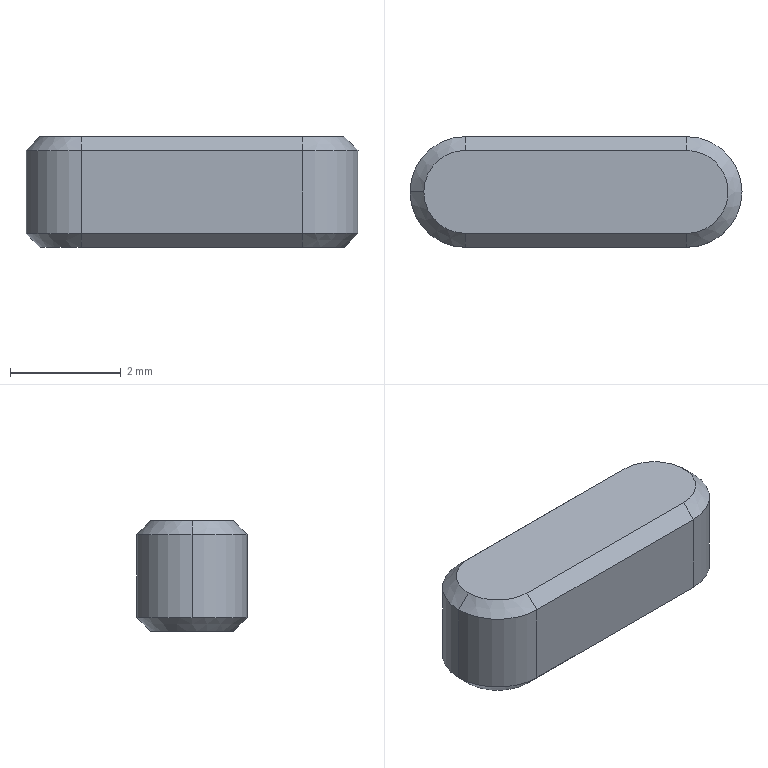Part | SolidWorks | features BaseBody 1 | 1 solid | 17 faces | box 6 x 2 x 2 mm | volume 21.423 mm3 | plane 8 | cone 6 | cylinder 3 | commonest cylinder face diameters 2 x3
STEP:
#1=CARTESIAN_POINT('',(-4.,-0.75,1.));
#2=VERTEX_POINT('',#1);
#3=CARTESIAN_POINT('',(-4.75,0.,1.));
#4=VERTEX_POINT('',#3);
#5=CARTESIAN_POINT('',(-4.,0.,1.));
#6=DIRECTION('',(0.,0.,-1.));
#7=DIRECTION('',(-1.,0.,0.));
#8=AXIS2_PLACEMENT_3D('',#5,#6,#7);
#9=CIRCLE('',#8,0.75);
#10=EDGE_CURVE('',#2,#4,#9,.T.);
#11=ORIENTED_EDGE('',*,*,#10,.T.);
#12=CARTESIAN_POINT('',(-5.,0.,0.75));
#13=VERTEX_POINT('',#12);
#14=CARTESIAN_POINT('',(-5.,0.,0.75));
#15=DIRECTION('',(-0.7071,0.,-0.7071));
#16=VECTOR('',#15,1000.);
#17=LINE('',#14,#16);
#18=EDGE_CURVE('',#4,#13,#17,.T.);
#19=ORIENTED_EDGE('',*,*,#18,.T.);
#20=CARTESIAN_POINT('',(-4.,-1.,0.75));
#21=VERTEX_POINT('',#20);
#22=CARTESIAN_POINT('',(-4.,0.,0.75));
#23=DIRECTION('',(0.,0.,1.));
#24=DIRECTION('',(-1.,0.,0.));
#25=AXIS2_PLACEMENT_3D('',#22,#23,#24);
#26=CIRCLE('',#25,1.);
#27=EDGE_CURVE('',#13,#21,#26,.T.);
#28=ORIENTED_EDGE('',*,*,#27,.T.);
#29=CARTESIAN_POINT('',(-4.,-498996.,-498994.25));
#30=DIRECTION('',(0.,0.7071,0.7071));
#31=VECTOR('',#30,1000.);
#32=LINE('',#29,#31);
#33=EDGE_CURVE('',#21,#2,#32,.T.);
#34=ORIENTED_EDGE('',*,*,#33,.T.);
#35=EDGE_LOOP('',(#11,#19,#28,#34));
#36=FACE_OUTER_BOUND('',#35,.T.);
#37=CARTESIAN_POINT('',(-4.,0.,0.75));
#38=DIRECTION('',(0.,0.,-1.));
#39=DIRECTION('',(-1.,0.,0.));
#40=AXIS2_PLACEMENT_3D('',#37,#38,#39);
#41=CONICAL_SURFACE('',#40,1.,0.7854);
#42=ADVANCED_FACE('',(#36),#41,.T.);
#43=ORIENTED_EDGE('',*,*,#27,.F.);
#44=CARTESIAN_POINT('',(-5.,0.,-0.75));
#45=VERTEX_POINT('',#44);
#46=CARTESIAN_POINT('',(-5.,0.,1.));
#47=DIRECTION('',(0.,0.,-1.));
#48=VECTOR('',#47,1000.);
#49=LINE('',#46,#48);
#50=EDGE_CURVE('',#13,#45,#49,.T.);
#51=ORIENTED_EDGE('',*,*,#50,.T.);
#52=CARTESIAN_POINT('',(-4.,-1.,-0.75));
#53=VERTEX_POINT('',#52);
#54=CARTESIAN_POINT('',(-4.,0.,-0.75));
#55=DIRECTION('',(0.,0.,-1.));
#56=DIRECTION('',(1.,0.,0.));
#57=AXIS2_PLACEMENT_3D('',#54,#55,#56);
#58=CIRCLE('',#57,1.);
#59=EDGE_CURVE('',#53,#45,#58,.T.);
#60=ORIENTED_EDGE('',*,*,#59,.F.);
#61=CARTESIAN_POINT('',(-4.,-1.,1.));
#62=DIRECTION('',(0.,0.,1.));
#63=VECTOR('',#62,1000.);
#64=LINE('',#61,#63);
#65=EDGE_CURVE('',#53,#21,#64,.T.);
#66=ORIENTED_EDGE('',*,*,#65,.T.);
#67=EDGE_LOOP('',(#43,#51,#60,#66));
#68=FACE_OUTER_BOUND('',#67,.T.);
#69=CARTESIAN_POINT('',(-4.,0.,1.));
#70=DIRECTION('',(0.,0.,-1.));
#71=DIRECTION('',(-1.,0.,0.));
#72=AXIS2_PLACEMENT_3D('',#69,#70,#71);
#73=CYLINDRICAL_SURFACE('',#72,1.);
#74=ADVANCED_FACE('',(#68),#73,.T.);
#75=CARTESIAN_POINT('',(0.,-0.75,-1.));
#76=VERTEX_POINT('',#75);
#77=CARTESIAN_POINT('',(0.75,0.,-1.));
#78=VERTEX_POINT('',#77);
#79=CARTESIAN_POINT('',(0.,0.,-1.));
#80=DIRECTION('',(0.,0.,1.));
#81=DIRECTION('',(1.,0.,0.));
#82=AXIS2_PLACEMENT_3D('',#79,#80,#81);
#83=CIRCLE('',#82,0.75);
#84=EDGE_CURVE('',#76,#78,#83,.T.);
#85=ORIENTED_EDGE('',*,*,#84,.T.);
#86=CARTESIAN_POINT('',(1.,0.,-0.75));
#87=VERTEX_POINT('',#86);
#88=CARTESIAN_POINT('',(1.,0.,-0.75));
#89=DIRECTION('',(0.7071,0.,0.7071));
#90=VECTOR('',#89,1000.);
#91=LINE('',#88,#90);
#92=EDGE_CURVE('',#78,#87,#91,.T.);
#93=ORIENTED_EDGE('',*,*,#92,.T.);
#94=CARTESIAN_POINT('',(0.,-1.,-0.75));
#95=VERTEX_POINT('',#94);
#96=CARTESIAN_POINT('',(0.,0.,-0.75));
#97=DIRECTION('',(0.,0.,1.));
#98=DIRECTION('',(-1.,0.,0.));
#99=AXIS2_PLACEMENT_3D('',#96,#97,#98);
#100=CIRCLE('',#99,1.);
#101=EDGE_CURVE('',#95,#87,#100,.T.);
#102=ORIENTED_EDGE('',*,*,#101,.F.);
#103=CARTESIAN_POINT('',(0.,-1.,-0.75));
#104=DIRECTION('',(0.,-0.7071,0.7071));
#105=VECTOR('',#104,1000.);
#106=LINE('',#103,#105);
#107=EDGE_CURVE('',#76,#95,#106,.T.);
#108=ORIENTED_EDGE('',*,*,#107,.F.);
#109=EDGE_LOOP('',(#85,#93,#102,#108));
#110=FACE_OUTER_BOUND('',#109,.T.);
#111=CARTESIAN_POINT('',(0.,0.,-0.75));
#112=DIRECTION('',(0.,0.,1.));
#113=DIRECTION('',(1.,0.,0.));
#114=AXIS2_PLACEMENT_3D('',#111,#112,#113);
#115=CONICAL_SURFACE('',#114,1.,0.7854);
#116=ADVANCED_FACE('',(#110),#115,.T.);
#117=ORIENTED_EDGE('',*,*,#10,.F.);
#118=CARTESIAN_POINT('',(0.,-0.75,1.));
#119=VERTEX_POINT('',#118);
#120=CARTESIAN_POINT('',(-4.,-0.75,1.));
#121=DIRECTION('',(-1.,0.,0.));
#122=VECTOR('',#121,1000.);
#123=LINE('',#120,#122);
#124=EDGE_CURVE('',#119,#2,#123,.T.);
#125=ORIENTED_EDGE('',*,*,#124,.F.);
#126=CARTESIAN_POINT('',(0.,0.75,1.));
#127=VERTEX_POINT('',#126);
#128=CARTESIAN_POINT('',(0.,0.,1.));
#129=DIRECTION('',(0.,0.,-1.));
#130=DIRECTION('',(-1.,0.,0.));
#131=AXIS2_PLACEMENT_3D('',#128,#129,#130);
#132=CIRCLE('',#131,0.75);
#133=EDGE_CURVE('',#127,#119,#132,.T.);
#134=ORIENTED_EDGE('',*,*,#133,.F.);
#135=CARTESIAN_POINT('',(-4.,0.75,1.));
#136=VERTEX_POINT('',#135);
#137=CARTESIAN_POINT('',(-4.,0.75,1.));
#138=DIRECTION('',(1.,0.,0.));
#139=VECTOR('',#138,1000.);
#140=LINE('',#137,#139);
#141=EDGE_CURVE('',#136,#127,#140,.T.);
#142=ORIENTED_EDGE('',*,*,#141,.F.);
#143=CARTESIAN_POINT('',(-4.,0.,1.));
#144=DIRECTION('',(0.,0.,-1.));
#145=DIRECTION('',(-1.,0.,0.));
#146=AXIS2_PLACEMENT_3D('',#143,#144,#145);
#147=CIRCLE('',#146,0.75);
#148=EDGE_CURVE('',#4,#136,#147,.T.);
#149=ORIENTED_EDGE('',*,*,#148,.F.);
#150=EDGE_LOOP('',(#117,#125,#134,#142,#149));
#151=FACE_OUTER_BOUND('',#150,.T.);
#152=CARTESIAN_POINT('',(-4.,0.,1.));
#153=DIRECTION('',(0.,0.,-1.));
#154=DIRECTION('',(-1.,0.,0.));
#155=AXIS2_PLACEMENT_3D('',#152,#153,#154);
#156=PLANE('',#155);
#157=ADVANCED_FACE('',(#151),#156,.F.);
#158=ORIENTED_EDGE('',*,*,#18,.F.);
#159=ORIENTED_EDGE('',*,*,#148,.T.);
#160=CARTESIAN_POINT('',(-4.,1.,0.75));
#161=VERTEX_POINT('',#160);
#162=CARTESIAN_POINT('',(-4.,498996.,-498994.25));
#163=DIRECTION('',(0.,0.7071,-0.7071));
#164=VECTOR('',#163,1000.);
#165=LINE('',#162,#164);
#166=EDGE_CURVE('',#136,#161,#165,.T.);
#167=ORIENTED_EDGE('',*,*,#166,.T.);
#168=CARTESIAN_POINT('',(-4.,0.,0.75));
#169=DIRECTION('',(0.,0.,1.));
#170=DIRECTION('',(-1.,0.,0.));
#171=AXIS2_PLACEMENT_3D('',#168,#169,#170);
#172=CIRCLE('',#171,1.);
#173=EDGE_CURVE('',#161,#13,#172,.T.);
#174=ORIENTED_EDGE('',*,*,#173,.T.);
#175=EDGE_LOOP('',(#158,#159,#167,#174));
#176=FACE_OUTER_BOUND('',#175,.T.);
#177=CARTESIAN_POINT('',(-4.,0.,0.75));
#178=DIRECTION('',(0.,0.,-1.));
#179=DIRECTION('',(-1.,0.,0.));
#180=AXIS2_PLACEMENT_3D('',#177,#178,#179);
#181=CONICAL_SURFACE('',#180,1.,0.7854);
#182=ADVANCED_FACE('',(#176),#181,.T.);
#183=CARTESIAN_POINT('',(0.,-1.,0.75));
#184=VERTEX_POINT('',#183);
#185=CARTESIAN_POINT('',(-4.,-1.,0.75));
#186=DIRECTION('',(-1.,0.,0.));
#187=VECTOR('',#186,1000.);
#188=LINE('',#185,#187);
#189=EDGE_CURVE('',#184,#21,#188,.T.);
#190=ORIENTED_EDGE('',*,*,#189,.F.);
#191=CARTESIAN_POINT('',(0.,-0.75,1.));
#192=DIRECTION('',(0.,-0.7071,-0.7071));
#193=VECTOR('',#192,1000.);
#194=LINE('',#191,#193);
#195=EDGE_CURVE('',#119,#184,#194,.T.);
#196=ORIENTED_EDGE('',*,*,#195,.F.);
#197=ORIENTED_EDGE('',*,*,#124,.T.);
#198=ORIENTED_EDGE('',*,*,#33,.F.);
#199=EDGE_LOOP('',(#190,#196,#197,#198));
#200=FACE_OUTER_BOUND('',#199,.T.);
#201=CARTESIAN_POINT('',(-4.,-0.75,1.));
#202=DIRECTION('',(0.,0.7071,-0.7071));
#203=DIRECTION('',(0.,0.7071,0.7071));
#204=AXIS2_PLACEMENT_3D('',#201,#202,#203);
#205=PLANE('',#204);
#206=ADVANCED_FACE('',(#200),#205,.F.);
#207=ORIENTED_EDGE('',*,*,#195,.T.);
#208=CARTESIAN_POINT('',(0.,1.,0.75));
#209=VERTEX_POINT('',#208);
#210=CARTESIAN_POINT('',(0.,0.,0.75));
#211=DIRECTION('',(0.,0.,1.));
#212=DIRECTION('',(-1.,0.,0.));
#213=AXIS2_PLACEMENT_3D('',#210,#211,#212);
#214=CIRCLE('',#213,1.);
#215=EDGE_CURVE('',#184,#209,#214,.T.);
#216=ORIENTED_EDGE('',*,*,#215,.T.);
#217=CARTESIAN_POINT('',(0.,499000.,-498998.25));
#218=DIRECTION('',(0.,-0.7071,0.7071));
#219=VECTOR('',#218,1000.);
#220=LINE('',#217,#219);
#221=EDGE_CURVE('',#209,#127,#220,.T.);
#222=ORIENTED_EDGE('',*,*,#221,.T.);
#223=ORIENTED_EDGE('',*,*,#133,.T.);
#224=EDGE_LOOP('',(#207,#216,#222,#223));
#225=FACE_OUTER_BOUND('',#224,.T.);
#226=CARTESIAN_POINT('',(0.,0.,0.75));
#227=DIRECTION('',(0.,0.,-1.));
#228=DIRECTION('',(-1.,0.,0.));
#229=AXIS2_PLACEMENT_3D('',#226,#227,#228);
#230=CONICAL_SURFACE('',#229,1.,0.7854);
#231=ADVANCED_FACE('',(#225),#230,.T.);
#232=CARTESIAN_POINT('',(-4.,1.,0.75));
#233=DIRECTION('',(1.,0.,0.));
#234=VECTOR('',#233,1000.);
#235=LINE('',#232,#234);
#236=EDGE_CURVE('',#161,#209,#235,.T.);
#237=ORIENTED_EDGE('',*,*,#236,.F.);
#238=ORIENTED_EDGE('',*,*,#166,.F.);
#239=ORIENTED_EDGE('',*,*,#141,.T.);
#240=ORIENTED_EDGE('',*,*,#221,.F.);
#241=EDGE_LOOP('',(#237,#238,#239,#240));
#242=FACE_OUTER_BOUND('',#241,.T.);
#243=CARTESIAN_POINT('',(-4.,0.75,1.));
#244=DIRECTION('',(0.,-0.7071,-0.7071));
#245=DIRECTION('',(0.,0.7071,-0.7071));
#246=AXIS2_PLACEMENT_3D('',#243,#244,#245);
#247=PLANE('',#246);
#248=ADVANCED_FACE('',(#242),#247,.F.);
#249=ORIENTED_EDGE('',*,*,#50,.F.);
#250=ORIENTED_EDGE('',*,*,#173,.F.);
#251=CARTESIAN_POINT('',(-4.,1.,-0.75));
#252=VERTEX_POINT('',#251);
#253=CARTESIAN_POINT('',(-4.,1.,1.));
#254=DIRECTION('',(0.,0.,-1.));
#255=VECTOR('',#254,1000.);
#256=LINE('',#253,#255);
#257=EDGE_CURVE('',#161,#252,#256,.T.);
#258=ORIENTED_EDGE('',*,*,#257,.T.);
#259=CARTESIAN_POINT('',(-4.,0.,-0.75));
#260=DIRECTION('',(0.,0.,-1.));
#261=DIRECTION('',(1.,0.,0.));
#262=AXIS2_PLACEMENT_3D('',#259,#260,#261);
#263=CIRCLE('',#262,1.);
#264=EDGE_CURVE('',#45,#252,#263,.T.);
#265=ORIENTED_EDGE('',*,*,#264,.F.);
#266=EDGE_LOOP('',(#249,#250,#258,#265));
#267=FACE_OUTER_BOUND('',#266,.T.);
#268=CARTESIAN_POINT('',(-4.,0.,1.));
#269=DIRECTION('',(0.,0.,-1.));
#270=DIRECTION('',(-1.,0.,0.));
#271=AXIS2_PLACEMENT_3D('',#268,#269,#270);
#272=CYLINDRICAL_SURFACE('',#271,1.);
#273=ADVANCED_FACE('',(#267),#272,.T.);
#274=CARTESIAN_POINT('',(0.,-1.,-0.75));
#275=DIRECTION('',(-1.,0.,0.));
#276=VECTOR('',#275,1000.);
#277=LINE('',#274,#276);
#278=EDGE_CURVE('',#95,#53,#277,.T.);
#279=ORIENTED_EDGE('',*,*,#278,.F.);
#280=CARTESIAN_POINT('',(0.,-1.,1.));
#281=DIRECTION('',(0.,0.,-1.));
#282=VECTOR('',#281,1000.);
#283=LINE('',#280,#282);
#284=EDGE_CURVE('',#184,#95,#283,.T.);
#285=ORIENTED_EDGE('',*,*,#284,.F.);
#286=ORIENTED_EDGE('',*,*,#189,.T.);
#287=ORIENTED_EDGE('',*,*,#65,.F.);
#288=EDGE_LOOP('',(#279,#285,#286,#287));
#289=FACE_OUTER_BOUND('',#288,.T.);
#290=CARTESIAN_POINT('',(0.,-1.,1.));
#291=DIRECTION('',(0.,1.,0.));
#292=DIRECTION('',(-1.,0.,0.));
#293=AXIS2_PLACEMENT_3D('',#290,#291,#292);
#294=PLANE('',#293);
#295=ADVANCED_FACE('',(#289),#294,.F.);
#296=ORIENTED_EDGE('',*,*,#284,.T.);
#297=ORIENTED_EDGE('',*,*,#101,.T.);
#298=CARTESIAN_POINT('',(0.,1.,-0.75));
#299=VERTEX_POINT('',#298);
#300=CARTESIAN_POINT('',(0.,0.,-0.75));
#301=DIRECTION('',(0.,0.,1.));
#302=DIRECTION('',(-1.,0.,0.));
#303=AXIS2_PLACEMENT_3D('',#300,#301,#302);
#304=CIRCLE('',#303,1.);
#305=EDGE_CURVE('',#87,#299,#304,.T.);
#306=ORIENTED_EDGE('',*,*,#305,.T.);
#307=CARTESIAN_POINT('',(0.,1.,1.));
#308=DIRECTION('',(0.,0.,1.));
#309=VECTOR('',#308,1000.);
#310=LINE('',#307,#309);
#311=EDGE_CURVE('',#299,#209,#310,.T.);
#312=ORIENTED_EDGE('',*,*,#311,.T.);
#313=ORIENTED_EDGE('',*,*,#215,.F.);
#314=EDGE_LOOP('',(#296,#297,#306,#312,#313));
#315=FACE_OUTER_BOUND('',#314,.T.);
#316=CARTESIAN_POINT('',(0.,0.,1.));
#317=DIRECTION('',(0.,0.,-1.));
#318=DIRECTION('',(-1.,0.,0.));
#319=AXIS2_PLACEMENT_3D('',#316,#317,#318);
#320=CYLINDRICAL_SURFACE('',#319,1.);
#321=ADVANCED_FACE('',(#315),#320,.T.);
#322=ORIENTED_EDGE('',*,*,#236,.T.);
#323=ORIENTED_EDGE('',*,*,#311,.F.);
#324=CARTESIAN_POINT('',(-4.,1.,-0.75));
#325=DIRECTION('',(1.,0.,0.));
#326=VECTOR('',#325,1000.);
#327=LINE('',#324,#326);
#328=EDGE_CURVE('',#252,#299,#327,.T.);
#329=ORIENTED_EDGE('',*,*,#328,.F.);
#330=ORIENTED_EDGE('',*,*,#257,.F.);
#331=EDGE_LOOP('',(#322,#323,#329,#330));
#332=FACE_OUTER_BOUND('',#331,.T.);
#333=CARTESIAN_POINT('',(-4.,1.,1.));
#334=DIRECTION('',(0.,-1.,0.));
#335=DIRECTION('',(0.,0.,-1.));
#336=AXIS2_PLACEMENT_3D('',#333,#334,#335);
#337=PLANE('',#336);
#338=ADVANCED_FACE('',(#332),#337,.F.);
#339=ORIENTED_EDGE('',*,*,#107,.T.);
#340=ORIENTED_EDGE('',*,*,#278,.T.);
#341=CARTESIAN_POINT('',(-4.,-0.75,-1.));
#342=VERTEX_POINT('',#341);
#343=CARTESIAN_POINT('',(-4.,-499001.75,499000.));
#344=DIRECTION('',(0.,-0.7071,0.7071));
#345=VECTOR('',#344,1000.);
#346=LINE('',#343,#345);
#347=EDGE_CURVE('',#342,#53,#346,.T.);
#348=ORIENTED_EDGE('',*,*,#347,.F.);
#349=CARTESIAN_POINT('',(0.,-0.75,-1.));
#350=DIRECTION('',(1.,0.,0.));
#351=VECTOR('',#350,1000.);
#352=LINE('',#349,#351);
#353=EDGE_CURVE('',#342,#76,#352,.T.);
#354=ORIENTED_EDGE('',*,*,#353,.T.);
#355=EDGE_LOOP('',(#339,#340,#348,#354));
#356=FACE_OUTER_BOUND('',#355,.T.);
#357=CARTESIAN_POINT('',(0.,-1.,-0.75));
#358=DIRECTION('',(0.,-0.7071,-0.7071));
#359=DIRECTION('',(0.,0.7071,-0.7071));
#360=AXIS2_PLACEMENT_3D('',#357,#358,#359);
#361=PLANE('',#360);
#362=ADVANCED_FACE('',(#356),#361,.T.);
#363=ORIENTED_EDGE('',*,*,#92,.F.);
#364=CARTESIAN_POINT('',(0.,0.75,-1.));
#365=VERTEX_POINT('',#364);
#366=CARTESIAN_POINT('',(0.,0.,-1.));
#367=DIRECTION('',(0.,0.,1.));
#368=DIRECTION('',(1.,0.,0.));
#369=AXIS2_PLACEMENT_3D('',#366,#367,#368);
#370=CIRCLE('',#369,0.75);
#371=EDGE_CURVE('',#78,#365,#370,.T.);
#372=ORIENTED_EDGE('',*,*,#371,.T.);
#373=CARTESIAN_POINT('',(0.,499000.,498998.25));
#374=DIRECTION('',(0.,0.7071,0.7071));
#375=VECTOR('',#374,1000.);
#376=LINE('',#373,#375);
#377=EDGE_CURVE('',#365,#299,#376,.T.);
#378=ORIENTED_EDGE('',*,*,#377,.T.);
#379=ORIENTED_EDGE('',*,*,#305,.F.);
#380=EDGE_LOOP('',(#363,#372,#378,#379));
#381=FACE_OUTER_BOUND('',#380,.T.);
#382=CARTESIAN_POINT('',(0.,0.,-0.75));
#383=DIRECTION('',(0.,0.,1.));
#384=DIRECTION('',(1.,0.,0.));
#385=AXIS2_PLACEMENT_3D('',#382,#383,#384);
#386=CONICAL_SURFACE('',#385,1.,0.7854);
#387=ADVANCED_FACE('',(#381),#386,.T.);
#388=CARTESIAN_POINT('',(-4.,0.75,-1.));
#389=VERTEX_POINT('',#388);
#390=CARTESIAN_POINT('',(-4.,499001.75,499000.));
#391=DIRECTION('',(0.,-0.7071,-0.7071));
#392=VECTOR('',#391,1000.);
#393=LINE('',#390,#392);
#394=EDGE_CURVE('',#252,#389,#393,.T.);
#395=ORIENTED_EDGE('',*,*,#394,.F.);
#396=ORIENTED_EDGE('',*,*,#328,.T.);
#397=ORIENTED_EDGE('',*,*,#377,.F.);
#398=CARTESIAN_POINT('',(-4.,0.75,-1.));
#399=DIRECTION('',(-1.,0.,0.));
#400=VECTOR('',#399,1000.);
#401=LINE('',#398,#400);
#402=EDGE_CURVE('',#365,#389,#401,.T.);
#403=ORIENTED_EDGE('',*,*,#402,.T.);
#404=EDGE_LOOP('',(#395,#396,#397,#403));
#405=FACE_OUTER_BOUND('',#404,.T.);
#406=CARTESIAN_POINT('',(-4.,1.,-0.75));
#407=DIRECTION('',(0.,0.7071,-0.7071));
#408=DIRECTION('',(0.,0.7071,0.7071));
#409=AXIS2_PLACEMENT_3D('',#406,#407,#408);
#410=PLANE('',#409);
#411=ADVANCED_FACE('',(#405),#410,.T.);
#412=CARTESIAN_POINT('',(-4.,0.,-1.));
#413=DIRECTION('',(0.,0.,-1.));
#414=DIRECTION('',(1.,0.,0.));
#415=AXIS2_PLACEMENT_3D('',#412,#413,#414);
#416=CIRCLE('',#415,0.75);
#417=EDGE_CURVE('',#342,#389,#416,.T.);
#418=ORIENTED_EDGE('',*,*,#417,.T.);
#419=ORIENTED_EDGE('',*,*,#402,.F.);
#420=ORIENTED_EDGE('',*,*,#371,.F.);
#421=ORIENTED_EDGE('',*,*,#84,.F.);
#422=ORIENTED_EDGE('',*,*,#353,.F.);
#423=EDGE_LOOP('',(#418,#419,#420,#421,#422));
#424=FACE_OUTER_BOUND('',#423,.T.);
#425=CARTESIAN_POINT('',(-4.,0.,-1.));
#426=DIRECTION('',(0.,0.,-1.));
#427=DIRECTION('',(-1.,0.,0.));
#428=AXIS2_PLACEMENT_3D('',#425,#426,#427);
#429=PLANE('',#428);
#430=ADVANCED_FACE('',(#424),#429,.T.);
#431=ORIENTED_EDGE('',*,*,#347,.T.);
#432=ORIENTED_EDGE('',*,*,#59,.T.);
#433=ORIENTED_EDGE('',*,*,#264,.T.);
#434=ORIENTED_EDGE('',*,*,#394,.T.);
#435=ORIENTED_EDGE('',*,*,#417,.F.);
#436=EDGE_LOOP('',(#431,#432,#433,#434,#435));
#437=FACE_OUTER_BOUND('',#436,.T.);
#438=CARTESIAN_POINT('',(-4.,0.,-0.75));
#439=DIRECTION('',(0.,0.,1.));
#440=DIRECTION('',(1.,0.,0.));
#441=AXIS2_PLACEMENT_3D('',#438,#439,#440);
#442=CONICAL_SURFACE('',#441,1.,0.7854);
#443=ADVANCED_FACE('',(#437),#442,.T.);
#444=CLOSED_SHELL('',(#42,#74,#116,#157,#182,#206,#231,#248,#273,#295,#321,#338,#362,#387,#411,#430,#443));
#445=MANIFOLD_SOLID_BREP('',#444);
#446=CARTESIAN_POINT('',(0.,0.,0.));
#447=DIRECTION('',(0.,0.,1.));
#448=DIRECTION('',(1.,0.,0.));
#449=AXIS2_PLACEMENT_3D('',#446,#447,#448);
#450=(LENGTH_UNIT()NAMED_UNIT(*)SI_UNIT(.MILLI.,.METRE.));
#451=UNCERTAINTY_MEASURE_WITH_UNIT(LENGTH_MEASURE(0.00001),#450,'','');
#452=(NAMED_UNIT(*)PLANE_ANGLE_UNIT()SI_UNIT($,.RADIAN.));
#453=(NAMED_UNIT(*)SI_UNIT($,.STERADIAN.)SOLID_ANGLE_UNIT());
#454=(GEOMETRIC_REPRESENTATION_CONTEXT(3)GLOBAL_UNCERTAINTY_ASSIGNED_CONTEXT((#451))GLOBAL_UNIT_ASSIGNED_CONTEXT((#450,#452,#453))REPRESENTATION_CONTEXT('',''));
#455=ADVANCED_BREP_SHAPE_REPRESENTATION('',(#445,#449),#454);